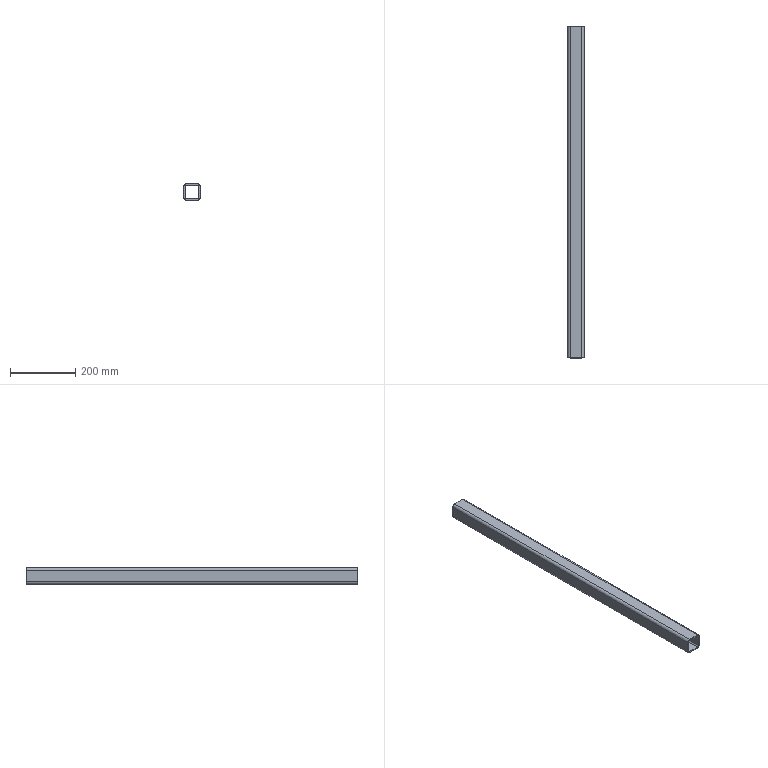Part | SolidWorks | features WeldMemberFeat 1, WeldmentFeature 1 | 1 solid | 18 faces | box 50 x 1020 x 50 mm | volume 708692 mm3 | plane 10 | cylinder 8 | commonest cylinder face diameters 8 x4 16 x4
STEP:
#1=CARTESIAN_POINT('',(-25.,0.,17.));
#2=VERTEX_POINT('',#1);
#3=CARTESIAN_POINT('',(-17.,0.,25.));
#4=VERTEX_POINT('',#3);
#5=CARTESIAN_POINT('',(-17.,0.,17.));
#6=DIRECTION('',(0.,1.,0.));
#7=DIRECTION('',(0.,0.,1.));
#8=AXIS2_PLACEMENT_3D('',#5,#6,#7);
#9=CIRCLE('',#8,8.);
#10=EDGE_CURVE('',#2,#4,#9,.T.);
#11=ORIENTED_EDGE('',*,*,#10,.T.);
#12=CARTESIAN_POINT('',(-17.,1020.,25.));
#13=VERTEX_POINT('',#12);
#14=CARTESIAN_POINT('',(-17.,1020.,25.));
#15=DIRECTION('',(0.,-1.,0.));
#16=VECTOR('',#15,1000.);
#17=LINE('',#14,#16);
#18=EDGE_CURVE('',#13,#4,#17,.T.);
#19=ORIENTED_EDGE('',*,*,#18,.F.);
#20=CARTESIAN_POINT('',(-25.,1020.,17.));
#21=VERTEX_POINT('',#20);
#22=CARTESIAN_POINT('',(-17.,1020.,17.));
#23=DIRECTION('',(0.,1.,0.));
#24=DIRECTION('',(0.,0.,1.));
#25=AXIS2_PLACEMENT_3D('',#22,#23,#24);
#26=CIRCLE('',#25,8.);
#27=EDGE_CURVE('',#21,#13,#26,.T.);
#28=ORIENTED_EDGE('',*,*,#27,.F.);
#29=CARTESIAN_POINT('',(-25.,1020.,17.));
#30=DIRECTION('',(0.,-1.,0.));
#31=VECTOR('',#30,1000.);
#32=LINE('',#29,#31);
#33=EDGE_CURVE('',#21,#2,#32,.T.);
#34=ORIENTED_EDGE('',*,*,#33,.T.);
#35=EDGE_LOOP('',(#11,#19,#28,#34));
#36=FACE_OUTER_BOUND('',#35,.T.);
#37=CARTESIAN_POINT('',(-17.,1020.,17.));
#38=DIRECTION('',(0.,-1.,0.));
#39=DIRECTION('',(0.,0.,-1.));
#40=AXIS2_PLACEMENT_3D('',#37,#38,#39);
#41=CYLINDRICAL_SURFACE('',#40,8.);
#42=ADVANCED_FACE('',(#36),#41,.T.);
#43=CARTESIAN_POINT('',(17.,0.,25.));
#44=VERTEX_POINT('',#43);
#45=CARTESIAN_POINT('',(-17.,0.,25.));
#46=DIRECTION('',(1.,0.,0.));
#47=VECTOR('',#46,1000.);
#48=LINE('',#45,#47);
#49=EDGE_CURVE('',#4,#44,#48,.T.);
#50=ORIENTED_EDGE('',*,*,#49,.T.);
#51=CARTESIAN_POINT('',(17.,1020.,25.));
#52=VERTEX_POINT('',#51);
#53=CARTESIAN_POINT('',(17.,1020.,25.));
#54=DIRECTION('',(0.,-1.,0.));
#55=VECTOR('',#54,1000.);
#56=LINE('',#53,#55);
#57=EDGE_CURVE('',#52,#44,#56,.T.);
#58=ORIENTED_EDGE('',*,*,#57,.F.);
#59=CARTESIAN_POINT('',(-17.,1020.,25.));
#60=DIRECTION('',(1.,0.,0.));
#61=VECTOR('',#60,1000.);
#62=LINE('',#59,#61);
#63=EDGE_CURVE('',#13,#52,#62,.T.);
#64=ORIENTED_EDGE('',*,*,#63,.F.);
#65=ORIENTED_EDGE('',*,*,#18,.T.);
#66=EDGE_LOOP('',(#50,#58,#64,#65));
#67=FACE_OUTER_BOUND('',#66,.T.);
#68=CARTESIAN_POINT('',(-17.,1020.,25.));
#69=DIRECTION('',(0.,0.,-1.));
#70=DIRECTION('',(-1.,0.,0.));
#71=AXIS2_PLACEMENT_3D('',#68,#69,#70);
#72=PLANE('',#71);
#73=ADVANCED_FACE('',(#67),#72,.F.);
#74=CARTESIAN_POINT('',(25.,0.,17.));
#75=VERTEX_POINT('',#74);
#76=CARTESIAN_POINT('',(17.,0.,17.));
#77=DIRECTION('',(0.,1.,0.));
#78=DIRECTION('',(0.,0.,1.));
#79=AXIS2_PLACEMENT_3D('',#76,#77,#78);
#80=CIRCLE('',#79,8.);
#81=EDGE_CURVE('',#44,#75,#80,.T.);
#82=ORIENTED_EDGE('',*,*,#81,.T.);
#83=CARTESIAN_POINT('',(25.,1020.,17.));
#84=VERTEX_POINT('',#83);
#85=CARTESIAN_POINT('',(25.,1020.,17.));
#86=DIRECTION('',(0.,-1.,0.));
#87=VECTOR('',#86,1000.);
#88=LINE('',#85,#87);
#89=EDGE_CURVE('',#84,#75,#88,.T.);
#90=ORIENTED_EDGE('',*,*,#89,.F.);
#91=CARTESIAN_POINT('',(17.,1020.,17.));
#92=DIRECTION('',(0.,1.,0.));
#93=DIRECTION('',(0.,0.,1.));
#94=AXIS2_PLACEMENT_3D('',#91,#92,#93);
#95=CIRCLE('',#94,8.);
#96=EDGE_CURVE('',#52,#84,#95,.T.);
#97=ORIENTED_EDGE('',*,*,#96,.F.);
#98=ORIENTED_EDGE('',*,*,#57,.T.);
#99=EDGE_LOOP('',(#82,#90,#97,#98));
#100=FACE_OUTER_BOUND('',#99,.T.);
#101=CARTESIAN_POINT('',(17.,1020.,17.));
#102=DIRECTION('',(0.,-1.,0.));
#103=DIRECTION('',(0.,0.,-1.));
#104=AXIS2_PLACEMENT_3D('',#101,#102,#103);
#105=CYLINDRICAL_SURFACE('',#104,8.);
#106=ADVANCED_FACE('',(#100),#105,.T.);
#107=CARTESIAN_POINT('',(25.,0.,-17.));
#108=VERTEX_POINT('',#107);
#109=CARTESIAN_POINT('',(25.,0.,-17.));
#110=DIRECTION('',(0.,0.,-1.));
#111=VECTOR('',#110,1000.);
#112=LINE('',#109,#111);
#113=EDGE_CURVE('',#75,#108,#112,.T.);
#114=ORIENTED_EDGE('',*,*,#113,.T.);
#115=CARTESIAN_POINT('',(25.,1020.,-17.));
#116=VERTEX_POINT('',#115);
#117=CARTESIAN_POINT('',(25.,1020.,-17.));
#118=DIRECTION('',(0.,-1.,0.));
#119=VECTOR('',#118,1000.);
#120=LINE('',#117,#119);
#121=EDGE_CURVE('',#116,#108,#120,.T.);
#122=ORIENTED_EDGE('',*,*,#121,.F.);
#123=CARTESIAN_POINT('',(25.,1020.,-17.));
#124=DIRECTION('',(0.,0.,-1.));
#125=VECTOR('',#124,1000.);
#126=LINE('',#123,#125);
#127=EDGE_CURVE('',#84,#116,#126,.T.);
#128=ORIENTED_EDGE('',*,*,#127,.F.);
#129=ORIENTED_EDGE('',*,*,#89,.T.);
#130=EDGE_LOOP('',(#114,#122,#128,#129));
#131=FACE_OUTER_BOUND('',#130,.T.);
#132=CARTESIAN_POINT('',(25.,1020.,-17.));
#133=DIRECTION('',(-1.,0.,0.));
#134=DIRECTION('',(0.,0.,1.));
#135=AXIS2_PLACEMENT_3D('',#132,#133,#134);
#136=PLANE('',#135);
#137=ADVANCED_FACE('',(#131),#136,.F.);
#138=CARTESIAN_POINT('',(17.,0.,-25.));
#139=VERTEX_POINT('',#138);
#140=CARTESIAN_POINT('',(17.,0.,-17.));
#141=DIRECTION('',(0.,1.,0.));
#142=DIRECTION('',(0.,0.,1.));
#143=AXIS2_PLACEMENT_3D('',#140,#141,#142);
#144=CIRCLE('',#143,8.);
#145=EDGE_CURVE('',#108,#139,#144,.T.);
#146=ORIENTED_EDGE('',*,*,#145,.T.);
#147=CARTESIAN_POINT('',(17.,1020.,-25.));
#148=VERTEX_POINT('',#147);
#149=CARTESIAN_POINT('',(17.,1020.,-25.));
#150=DIRECTION('',(0.,-1.,0.));
#151=VECTOR('',#150,1000.);
#152=LINE('',#149,#151);
#153=EDGE_CURVE('',#148,#139,#152,.T.);
#154=ORIENTED_EDGE('',*,*,#153,.F.);
#155=CARTESIAN_POINT('',(17.,1020.,-17.));
#156=DIRECTION('',(0.,1.,0.));
#157=DIRECTION('',(0.,0.,1.));
#158=AXIS2_PLACEMENT_3D('',#155,#156,#157);
#159=CIRCLE('',#158,8.);
#160=EDGE_CURVE('',#116,#148,#159,.T.);
#161=ORIENTED_EDGE('',*,*,#160,.F.);
#162=ORIENTED_EDGE('',*,*,#121,.T.);
#163=EDGE_LOOP('',(#146,#154,#161,#162));
#164=FACE_OUTER_BOUND('',#163,.T.);
#165=CARTESIAN_POINT('',(17.,1020.,-17.));
#166=DIRECTION('',(0.,-1.,0.));
#167=DIRECTION('',(0.,0.,-1.));
#168=AXIS2_PLACEMENT_3D('',#165,#166,#167);
#169=CYLINDRICAL_SURFACE('',#168,8.);
#170=ADVANCED_FACE('',(#164),#169,.T.);
#171=CARTESIAN_POINT('',(-17.,0.,-25.));
#172=VERTEX_POINT('',#171);
#173=CARTESIAN_POINT('',(17.,0.,-25.));
#174=DIRECTION('',(-1.,0.,0.));
#175=VECTOR('',#174,1000.);
#176=LINE('',#173,#175);
#177=EDGE_CURVE('',#139,#172,#176,.T.);
#178=ORIENTED_EDGE('',*,*,#177,.T.);
#179=CARTESIAN_POINT('',(-17.,1020.,-25.));
#180=VERTEX_POINT('',#179);
#181=CARTESIAN_POINT('',(-17.,1020.,-25.));
#182=DIRECTION('',(0.,-1.,0.));
#183=VECTOR('',#182,1000.);
#184=LINE('',#181,#183);
#185=EDGE_CURVE('',#180,#172,#184,.T.);
#186=ORIENTED_EDGE('',*,*,#185,.F.);
#187=CARTESIAN_POINT('',(17.,1020.,-25.));
#188=DIRECTION('',(-1.,0.,0.));
#189=VECTOR('',#188,1000.);
#190=LINE('',#187,#189);
#191=EDGE_CURVE('',#148,#180,#190,.T.);
#192=ORIENTED_EDGE('',*,*,#191,.F.);
#193=ORIENTED_EDGE('',*,*,#153,.T.);
#194=EDGE_LOOP('',(#178,#186,#192,#193));
#195=FACE_OUTER_BOUND('',#194,.T.);
#196=CARTESIAN_POINT('',(17.,1020.,-25.));
#197=DIRECTION('',(0.,0.,1.));
#198=DIRECTION('',(1.,0.,0.));
#199=AXIS2_PLACEMENT_3D('',#196,#197,#198);
#200=PLANE('',#199);
#201=ADVANCED_FACE('',(#195),#200,.F.);
#202=CARTESIAN_POINT('',(-25.,0.,-17.));
#203=VERTEX_POINT('',#202);
#204=CARTESIAN_POINT('',(-17.,0.,-17.));
#205=DIRECTION('',(0.,1.,0.));
#206=DIRECTION('',(0.,0.,1.));
#207=AXIS2_PLACEMENT_3D('',#204,#205,#206);
#208=CIRCLE('',#207,8.);
#209=EDGE_CURVE('',#172,#203,#208,.T.);
#210=ORIENTED_EDGE('',*,*,#209,.T.);
#211=CARTESIAN_POINT('',(-25.,1020.,-17.));
#212=VERTEX_POINT('',#211);
#213=CARTESIAN_POINT('',(-25.,1020.,-17.));
#214=DIRECTION('',(0.,-1.,0.));
#215=VECTOR('',#214,1000.);
#216=LINE('',#213,#215);
#217=EDGE_CURVE('',#212,#203,#216,.T.);
#218=ORIENTED_EDGE('',*,*,#217,.F.);
#219=CARTESIAN_POINT('',(-17.,1020.,-17.));
#220=DIRECTION('',(0.,1.,0.));
#221=DIRECTION('',(0.,0.,1.));
#222=AXIS2_PLACEMENT_3D('',#219,#220,#221);
#223=CIRCLE('',#222,8.);
#224=EDGE_CURVE('',#180,#212,#223,.T.);
#225=ORIENTED_EDGE('',*,*,#224,.F.);
#226=ORIENTED_EDGE('',*,*,#185,.T.);
#227=EDGE_LOOP('',(#210,#218,#225,#226));
#228=FACE_OUTER_BOUND('',#227,.T.);
#229=CARTESIAN_POINT('',(-17.,1020.,-17.));
#230=DIRECTION('',(0.,-1.,0.));
#231=DIRECTION('',(0.,0.,-1.));
#232=AXIS2_PLACEMENT_3D('',#229,#230,#231);
#233=CYLINDRICAL_SURFACE('',#232,8.);
#234=ADVANCED_FACE('',(#228),#233,.T.);
#235=CARTESIAN_POINT('',(17.,0.,21.));
#236=VERTEX_POINT('',#235);
#237=CARTESIAN_POINT('',(21.,0.,17.));
#238=VERTEX_POINT('',#237);
#239=CARTESIAN_POINT('',(17.,0.,17.));
#240=DIRECTION('',(0.,1.,0.));
#241=DIRECTION('',(0.,0.,1.));
#242=AXIS2_PLACEMENT_3D('',#239,#240,#241);
#243=CIRCLE('',#242,4.);
#244=EDGE_CURVE('',#236,#238,#243,.T.);
#245=ORIENTED_EDGE('',*,*,#244,.F.);
#246=CARTESIAN_POINT('',(17.,1020.,21.));
#247=VERTEX_POINT('',#246);
#248=CARTESIAN_POINT('',(17.,1020.,21.));
#249=DIRECTION('',(0.,-1.,0.));
#250=VECTOR('',#249,1000.);
#251=LINE('',#248,#250);
#252=EDGE_CURVE('',#247,#236,#251,.T.);
#253=ORIENTED_EDGE('',*,*,#252,.F.);
#254=CARTESIAN_POINT('',(21.,1020.,17.));
#255=VERTEX_POINT('',#254);
#256=CARTESIAN_POINT('',(17.,1020.,17.));
#257=DIRECTION('',(0.,1.,0.));
#258=DIRECTION('',(0.,0.,1.));
#259=AXIS2_PLACEMENT_3D('',#256,#257,#258);
#260=CIRCLE('',#259,4.);
#261=EDGE_CURVE('',#247,#255,#260,.T.);
#262=ORIENTED_EDGE('',*,*,#261,.T.);
#263=CARTESIAN_POINT('',(21.,1020.,17.));
#264=DIRECTION('',(0.,-1.,0.));
#265=VECTOR('',#264,1000.);
#266=LINE('',#263,#265);
#267=EDGE_CURVE('',#255,#238,#266,.T.);
#268=ORIENTED_EDGE('',*,*,#267,.T.);
#269=EDGE_LOOP('',(#245,#253,#262,#268));
#270=FACE_OUTER_BOUND('',#269,.T.);
#271=CARTESIAN_POINT('',(17.,1020.,17.));
#272=DIRECTION('',(0.,-1.,0.));
#273=DIRECTION('',(0.,0.,-1.));
#274=AXIS2_PLACEMENT_3D('',#271,#272,#273);
#275=CYLINDRICAL_SURFACE('',#274,4.);
#276=ADVANCED_FACE('',(#270),#275,.F.);
#277=CARTESIAN_POINT('',(-17.,0.,21.));
#278=VERTEX_POINT('',#277);
#279=CARTESIAN_POINT('',(-17.,0.,21.));
#280=DIRECTION('',(1.,0.,0.));
#281=VECTOR('',#280,1000.);
#282=LINE('',#279,#281);
#283=EDGE_CURVE('',#278,#236,#282,.T.);
#284=ORIENTED_EDGE('',*,*,#283,.F.);
#285=CARTESIAN_POINT('',(-17.,1020.,21.));
#286=VERTEX_POINT('',#285);
#287=CARTESIAN_POINT('',(-17.,1020.,21.));
#288=DIRECTION('',(0.,-1.,0.));
#289=VECTOR('',#288,1000.);
#290=LINE('',#287,#289);
#291=EDGE_CURVE('',#286,#278,#290,.T.);
#292=ORIENTED_EDGE('',*,*,#291,.F.);
#293=CARTESIAN_POINT('',(-17.,1020.,21.));
#294=DIRECTION('',(1.,0.,0.));
#295=VECTOR('',#294,1000.);
#296=LINE('',#293,#295);
#297=EDGE_CURVE('',#286,#247,#296,.T.);
#298=ORIENTED_EDGE('',*,*,#297,.T.);
#299=ORIENTED_EDGE('',*,*,#252,.T.);
#300=EDGE_LOOP('',(#284,#292,#298,#299));
#301=FACE_OUTER_BOUND('',#300,.T.);
#302=CARTESIAN_POINT('',(-17.,1020.,21.));
#303=DIRECTION('',(0.,0.,-1.));
#304=DIRECTION('',(-1.,0.,0.));
#305=AXIS2_PLACEMENT_3D('',#302,#303,#304);
#306=PLANE('',#305);
#307=ADVANCED_FACE('',(#301),#306,.T.);
#308=CARTESIAN_POINT('',(-21.,0.,17.));
#309=VERTEX_POINT('',#308);
#310=CARTESIAN_POINT('',(-17.,0.,17.));
#311=DIRECTION('',(0.,1.,0.));
#312=DIRECTION('',(0.,0.,1.));
#313=AXIS2_PLACEMENT_3D('',#310,#311,#312);
#314=CIRCLE('',#313,4.);
#315=EDGE_CURVE('',#309,#278,#314,.T.);
#316=ORIENTED_EDGE('',*,*,#315,.F.);
#317=CARTESIAN_POINT('',(-21.,1020.,17.));
#318=VERTEX_POINT('',#317);
#319=CARTESIAN_POINT('',(-21.,1020.,17.));
#320=DIRECTION('',(0.,-1.,0.));
#321=VECTOR('',#320,1000.);
#322=LINE('',#319,#321);
#323=EDGE_CURVE('',#318,#309,#322,.T.);
#324=ORIENTED_EDGE('',*,*,#323,.F.);
#325=CARTESIAN_POINT('',(-17.,1020.,17.));
#326=DIRECTION('',(0.,1.,0.));
#327=DIRECTION('',(0.,0.,1.));
#328=AXIS2_PLACEMENT_3D('',#325,#326,#327);
#329=CIRCLE('',#328,4.);
#330=EDGE_CURVE('',#318,#286,#329,.T.);
#331=ORIENTED_EDGE('',*,*,#330,.T.);
#332=ORIENTED_EDGE('',*,*,#291,.T.);
#333=EDGE_LOOP('',(#316,#324,#331,#332));
#334=FACE_OUTER_BOUND('',#333,.T.);
#335=CARTESIAN_POINT('',(-17.,1020.,17.));
#336=DIRECTION('',(0.,-1.,0.));
#337=DIRECTION('',(0.,0.,-1.));
#338=AXIS2_PLACEMENT_3D('',#335,#336,#337);
#339=CYLINDRICAL_SURFACE('',#338,4.);
#340=ADVANCED_FACE('',(#334),#339,.F.);
#341=CARTESIAN_POINT('',(-21.,0.,-17.));
#342=VERTEX_POINT('',#341);
#343=CARTESIAN_POINT('',(-21.,0.,17.));
#344=DIRECTION('',(0.,0.,1.));
#345=VECTOR('',#344,1000.);
#346=LINE('',#343,#345);
#347=EDGE_CURVE('',#342,#309,#346,.T.);
#348=ORIENTED_EDGE('',*,*,#347,.F.);
#349=CARTESIAN_POINT('',(-21.,1020.,-17.));
#350=VERTEX_POINT('',#349);
#351=CARTESIAN_POINT('',(-21.,1020.,-17.));
#352=DIRECTION('',(0.,-1.,0.));
#353=VECTOR('',#352,1000.);
#354=LINE('',#351,#353);
#355=EDGE_CURVE('',#350,#342,#354,.T.);
#356=ORIENTED_EDGE('',*,*,#355,.F.);
#357=CARTESIAN_POINT('',(-21.,1020.,17.));
#358=DIRECTION('',(0.,0.,1.));
#359=VECTOR('',#358,1000.);
#360=LINE('',#357,#359);
#361=EDGE_CURVE('',#350,#318,#360,.T.);
#362=ORIENTED_EDGE('',*,*,#361,.T.);
#363=ORIENTED_EDGE('',*,*,#323,.T.);
#364=EDGE_LOOP('',(#348,#356,#362,#363));
#365=FACE_OUTER_BOUND('',#364,.T.);
#366=CARTESIAN_POINT('',(-21.,1020.,17.));
#367=DIRECTION('',(1.,0.,0.));
#368=DIRECTION('',(0.,0.,-1.));
#369=AXIS2_PLACEMENT_3D('',#366,#367,#368);
#370=PLANE('',#369);
#371=ADVANCED_FACE('',(#365),#370,.T.);
#372=CARTESIAN_POINT('',(-17.,0.,-21.));
#373=VERTEX_POINT('',#372);
#374=CARTESIAN_POINT('',(-17.,0.,-17.));
#375=DIRECTION('',(0.,1.,0.));
#376=DIRECTION('',(0.,0.,1.));
#377=AXIS2_PLACEMENT_3D('',#374,#375,#376);
#378=CIRCLE('',#377,4.);
#379=EDGE_CURVE('',#373,#342,#378,.T.);
#380=ORIENTED_EDGE('',*,*,#379,.F.);
#381=CARTESIAN_POINT('',(-17.,1020.,-21.));
#382=VERTEX_POINT('',#381);
#383=CARTESIAN_POINT('',(-17.,1020.,-21.));
#384=DIRECTION('',(0.,-1.,0.));
#385=VECTOR('',#384,1000.);
#386=LINE('',#383,#385);
#387=EDGE_CURVE('',#382,#373,#386,.T.);
#388=ORIENTED_EDGE('',*,*,#387,.F.);
#389=CARTESIAN_POINT('',(-17.,1020.,-17.));
#390=DIRECTION('',(0.,1.,0.));
#391=DIRECTION('',(0.,0.,1.));
#392=AXIS2_PLACEMENT_3D('',#389,#390,#391);
#393=CIRCLE('',#392,4.);
#394=EDGE_CURVE('',#382,#350,#393,.T.);
#395=ORIENTED_EDGE('',*,*,#394,.T.);
#396=ORIENTED_EDGE('',*,*,#355,.T.);
#397=EDGE_LOOP('',(#380,#388,#395,#396));
#398=FACE_OUTER_BOUND('',#397,.T.);
#399=CARTESIAN_POINT('',(-17.,1020.,-17.));
#400=DIRECTION('',(0.,-1.,0.));
#401=DIRECTION('',(0.,0.,-1.));
#402=AXIS2_PLACEMENT_3D('',#399,#400,#401);
#403=CYLINDRICAL_SURFACE('',#402,4.);
#404=ADVANCED_FACE('',(#398),#403,.F.);
#405=CARTESIAN_POINT('',(17.,0.,-21.));
#406=VERTEX_POINT('',#405);
#407=CARTESIAN_POINT('',(17.,0.,-21.));
#408=DIRECTION('',(-1.,0.,0.));
#409=VECTOR('',#408,1000.);
#410=LINE('',#407,#409);
#411=EDGE_CURVE('',#406,#373,#410,.T.);
#412=ORIENTED_EDGE('',*,*,#411,.F.);
#413=CARTESIAN_POINT('',(17.,1020.,-21.));
#414=VERTEX_POINT('',#413);
#415=CARTESIAN_POINT('',(17.,1020.,-21.));
#416=DIRECTION('',(0.,-1.,0.));
#417=VECTOR('',#416,1000.);
#418=LINE('',#415,#417);
#419=EDGE_CURVE('',#414,#406,#418,.T.);
#420=ORIENTED_EDGE('',*,*,#419,.F.);
#421=CARTESIAN_POINT('',(17.,1020.,-21.));
#422=DIRECTION('',(-1.,0.,0.));
#423=VECTOR('',#422,1000.);
#424=LINE('',#421,#423);
#425=EDGE_CURVE('',#414,#382,#424,.T.);
#426=ORIENTED_EDGE('',*,*,#425,.T.);
#427=ORIENTED_EDGE('',*,*,#387,.T.);
#428=EDGE_LOOP('',(#412,#420,#426,#427));
#429=FACE_OUTER_BOUND('',#428,.T.);
#430=CARTESIAN_POINT('',(17.,1020.,-21.));
#431=DIRECTION('',(0.,0.,1.));
#432=DIRECTION('',(1.,0.,0.));
#433=AXIS2_PLACEMENT_3D('',#430,#431,#432);
#434=PLANE('',#433);
#435=ADVANCED_FACE('',(#429),#434,.T.);
#436=CARTESIAN_POINT('',(21.,0.,-17.));
#437=VERTEX_POINT('',#436);
#438=CARTESIAN_POINT('',(17.,0.,-17.));
#439=DIRECTION('',(0.,1.,0.));
#440=DIRECTION('',(0.,0.,1.));
#441=AXIS2_PLACEMENT_3D('',#438,#439,#440);
#442=CIRCLE('',#441,4.);
#443=EDGE_CURVE('',#437,#406,#442,.T.);
#444=ORIENTED_EDGE('',*,*,#443,.F.);
#445=CARTESIAN_POINT('',(21.,1020.,-17.));
#446=VERTEX_POINT('',#445);
#447=CARTESIAN_POINT('',(21.,1020.,-17.));
#448=DIRECTION('',(0.,-1.,0.));
#449=VECTOR('',#448,1000.);
#450=LINE('',#447,#449);
#451=EDGE_CURVE('',#446,#437,#450,.T.);
#452=ORIENTED_EDGE('',*,*,#451,.F.);
#453=CARTESIAN_POINT('',(17.,1020.,-17.));
#454=DIRECTION('',(0.,1.,0.));
#455=DIRECTION('',(0.,0.,1.));
#456=AXIS2_PLACEMENT_3D('',#453,#454,#455);
#457=CIRCLE('',#456,4.);
#458=EDGE_CURVE('',#446,#414,#457,.T.);
#459=ORIENTED_EDGE('',*,*,#458,.T.);
#460=ORIENTED_EDGE('',*,*,#419,.T.);
#461=EDGE_LOOP('',(#444,#452,#459,#460));
#462=FACE_OUTER_BOUND('',#461,.T.);
#463=CARTESIAN_POINT('',(17.,1020.,-17.));
#464=DIRECTION('',(0.,-1.,0.));
#465=DIRECTION('',(0.,0.,-1.));
#466=AXIS2_PLACEMENT_3D('',#463,#464,#465);
#467=CYLINDRICAL_SURFACE('',#466,4.);
#468=ADVANCED_FACE('',(#462),#467,.F.);
#469=CARTESIAN_POINT('',(21.,0.,-17.));
#470=DIRECTION('',(0.,0.,-1.));
#471=VECTOR('',#470,1000.);
#472=LINE('',#469,#471);
#473=EDGE_CURVE('',#238,#437,#472,.T.);
#474=ORIENTED_EDGE('',*,*,#473,.F.);
#475=ORIENTED_EDGE('',*,*,#267,.F.);
#476=CARTESIAN_POINT('',(21.,1020.,-17.));
#477=DIRECTION('',(0.,0.,-1.));
#478=VECTOR('',#477,1000.);
#479=LINE('',#476,#478);
#480=EDGE_CURVE('',#255,#446,#479,.T.);
#481=ORIENTED_EDGE('',*,*,#480,.T.);
#482=ORIENTED_EDGE('',*,*,#451,.T.);
#483=EDGE_LOOP('',(#474,#475,#481,#482));
#484=FACE_OUTER_BOUND('',#483,.T.);
#485=CARTESIAN_POINT('',(21.,1020.,-17.));
#486=DIRECTION('',(-1.,0.,0.));
#487=DIRECTION('',(0.,0.,1.));
#488=AXIS2_PLACEMENT_3D('',#485,#486,#487);
#489=PLANE('',#488);
#490=ADVANCED_FACE('',(#484),#489,.T.);
#491=CARTESIAN_POINT('',(-25.,0.,17.));
#492=DIRECTION('',(0.,0.,1.));
#493=VECTOR('',#492,1000.);
#494=LINE('',#491,#493);
#495=EDGE_CURVE('',#203,#2,#494,.T.);
#496=ORIENTED_EDGE('',*,*,#495,.T.);
#497=ORIENTED_EDGE('',*,*,#33,.F.);
#498=CARTESIAN_POINT('',(-25.,1020.,17.));
#499=DIRECTION('',(0.,0.,1.));
#500=VECTOR('',#499,1000.);
#501=LINE('',#498,#500);
#502=EDGE_CURVE('',#212,#21,#501,.T.);
#503=ORIENTED_EDGE('',*,*,#502,.F.);
#504=ORIENTED_EDGE('',*,*,#217,.T.);
#505=EDGE_LOOP('',(#496,#497,#503,#504));
#506=FACE_OUTER_BOUND('',#505,.T.);
#507=CARTESIAN_POINT('',(-25.,1020.,17.));
#508=DIRECTION('',(1.,0.,0.));
#509=DIRECTION('',(0.,0.,-1.));
#510=AXIS2_PLACEMENT_3D('',#507,#508,#509);
#511=PLANE('',#510);
#512=ADVANCED_FACE('',(#506),#511,.F.);
#513=ORIENTED_EDGE('',*,*,#261,.F.);
#514=ORIENTED_EDGE('',*,*,#297,.F.);
#515=ORIENTED_EDGE('',*,*,#330,.F.);
#516=ORIENTED_EDGE('',*,*,#361,.F.);
#517=ORIENTED_EDGE('',*,*,#394,.F.);
#518=ORIENTED_EDGE('',*,*,#425,.F.);
#519=ORIENTED_EDGE('',*,*,#458,.F.);
#520=ORIENTED_EDGE('',*,*,#480,.F.);
#521=EDGE_LOOP('',(#513,#514,#515,#516,#517,#518,#519,#520));
#522=FACE_BOUND('',#521,.T.);
#523=ORIENTED_EDGE('',*,*,#27,.T.);
#524=ORIENTED_EDGE('',*,*,#63,.T.);
#525=ORIENTED_EDGE('',*,*,#96,.T.);
#526=ORIENTED_EDGE('',*,*,#127,.T.);
#527=ORIENTED_EDGE('',*,*,#160,.T.);
#528=ORIENTED_EDGE('',*,*,#191,.T.);
#529=ORIENTED_EDGE('',*,*,#224,.T.);
#530=ORIENTED_EDGE('',*,*,#502,.T.);
#531=EDGE_LOOP('',(#523,#524,#525,#526,#527,#528,#529,#530));
#532=FACE_OUTER_BOUND('',#531,.T.);
#533=CARTESIAN_POINT('',(-17.,1020.,17.));
#534=DIRECTION('',(0.,1.,0.));
#535=DIRECTION('',(0.,0.,1.));
#536=AXIS2_PLACEMENT_3D('',#533,#534,#535);
#537=PLANE('',#536);
#538=ADVANCED_FACE('',(#522,#532),#537,.T.);
#539=ORIENTED_EDGE('',*,*,#244,.T.);
#540=ORIENTED_EDGE('',*,*,#473,.T.);
#541=ORIENTED_EDGE('',*,*,#443,.T.);
#542=ORIENTED_EDGE('',*,*,#411,.T.);
#543=ORIENTED_EDGE('',*,*,#379,.T.);
#544=ORIENTED_EDGE('',*,*,#347,.T.);
#545=ORIENTED_EDGE('',*,*,#315,.T.);
#546=ORIENTED_EDGE('',*,*,#283,.T.);
#547=EDGE_LOOP('',(#539,#540,#541,#542,#543,#544,#545,#546));
#548=FACE_BOUND('',#547,.T.);
#549=ORIENTED_EDGE('',*,*,#10,.F.);
#550=ORIENTED_EDGE('',*,*,#495,.F.);
#551=ORIENTED_EDGE('',*,*,#209,.F.);
#552=ORIENTED_EDGE('',*,*,#177,.F.);
#553=ORIENTED_EDGE('',*,*,#145,.F.);
#554=ORIENTED_EDGE('',*,*,#113,.F.);
#555=ORIENTED_EDGE('',*,*,#81,.F.);
#556=ORIENTED_EDGE('',*,*,#49,.F.);
#557=EDGE_LOOP('',(#549,#550,#551,#552,#553,#554,#555,#556));
#558=FACE_OUTER_BOUND('',#557,.T.);
#559=CARTESIAN_POINT('',(-17.,0.,17.));
#560=DIRECTION('',(0.,1.,0.));
#561=DIRECTION('',(0.,0.,1.));
#562=AXIS2_PLACEMENT_3D('',#559,#560,#561);
#563=PLANE('',#562);
#564=ADVANCED_FACE('',(#548,#558),#563,.F.);
#565=CLOSED_SHELL('',(#42,#73,#106,#137,#170,#201,#234,#276,#307,#340,#371,#404,#435,#468,#490,#512,#538,#564));
#566=MANIFOLD_SOLID_BREP('',#565);
#567=CARTESIAN_POINT('',(0.,0.,0.));
#568=DIRECTION('',(0.,0.,1.));
#569=DIRECTION('',(1.,0.,0.));
#570=AXIS2_PLACEMENT_3D('',#567,#568,#569);
#571=(LENGTH_UNIT()NAMED_UNIT(*)SI_UNIT(.MILLI.,.METRE.));
#572=UNCERTAINTY_MEASURE_WITH_UNIT(LENGTH_MEASURE(0.00001),#571,'','');
#573=(NAMED_UNIT(*)PLANE_ANGLE_UNIT()SI_UNIT($,.RADIAN.));
#574=(NAMED_UNIT(*)SI_UNIT($,.STERADIAN.)SOLID_ANGLE_UNIT());
#575=(GEOMETRIC_REPRESENTATION_CONTEXT(3)GLOBAL_UNCERTAINTY_ASSIGNED_CONTEXT((#572))GLOBAL_UNIT_ASSIGNED_CONTEXT((#571,#573,#574))REPRESENTATION_CONTEXT('',''));
#576=ADVANCED_BREP_SHAPE_REPRESENTATION('',(#566,#570),#575);